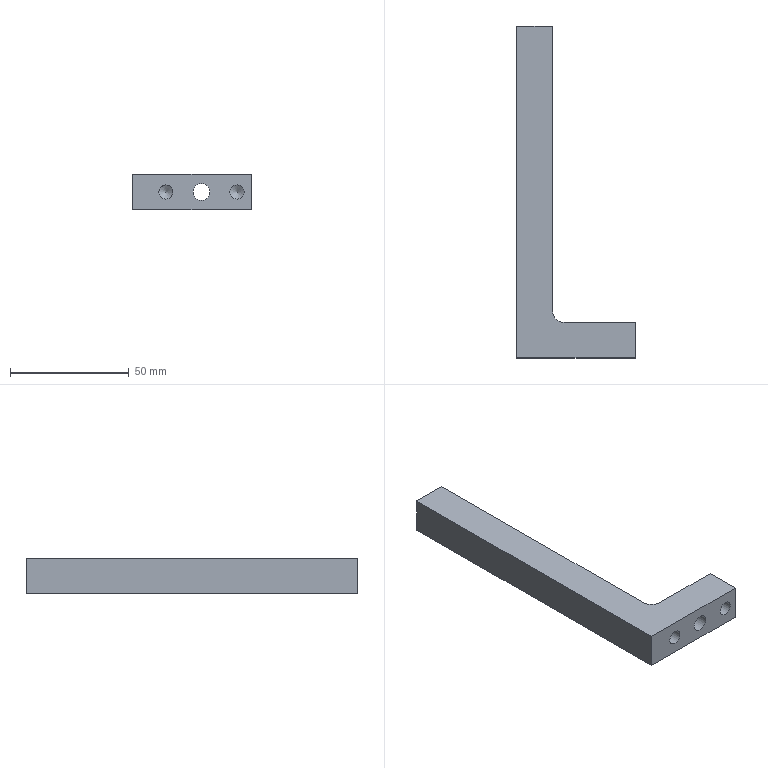Part | NX | features BREP 1 | 1 solid | 16 faces | box 50 x 140 x 15 mm | volume 37424 mm3 | plane 8 | cylinder 5 | cone 3 | commonest cylinder face diameters 6 x2 6.8 x1 7 x1 10 x1
STEP:
#1=CARTESIAN_POINT('',(15.,20.,0.));
#2=VERTEX_POINT('',#1);
#3=CARTESIAN_POINT('',(15.,140.,0.));
#4=VERTEX_POINT('',#3);
#5=CARTESIAN_POINT('',(15.,0.,0.));
#6=DIRECTION('',(0.,1.,0.));
#7=VECTOR('',#6,1000.);
#8=LINE('',#5,#7);
#9=EDGE_CURVE('',#2,#4,#8,.T.);
#10=ORIENTED_EDGE('',*,*,#9,.F.);
#11=CARTESIAN_POINT('',(20.,15.,0.));
#12=VERTEX_POINT('',#11);
#13=CARTESIAN_POINT('',(20.,20.,0.));
#14=DIRECTION('',(0.,0.,-1.));
#15=DIRECTION('',(1.,0.,0.));
#16=AXIS2_PLACEMENT_3D('',#13,#14,#15);
#17=CIRCLE('',#16,5.);
#18=EDGE_CURVE('',#12,#2,#17,.T.);
#19=ORIENTED_EDGE('',*,*,#18,.F.);
#20=CARTESIAN_POINT('',(50.,15.,0.));
#21=VERTEX_POINT('',#20);
#22=CARTESIAN_POINT('',(0.,15.,0.));
#23=DIRECTION('',(-1.,0.,0.));
#24=VECTOR('',#23,1000.);
#25=LINE('',#22,#24);
#26=EDGE_CURVE('',#21,#12,#25,.T.);
#27=ORIENTED_EDGE('',*,*,#26,.F.);
#28=CARTESIAN_POINT('',(50.,0.,0.));
#29=VERTEX_POINT('',#28);
#30=CARTESIAN_POINT('',(50.,0.,0.));
#31=DIRECTION('',(0.,1.,0.));
#32=VECTOR('',#31,1000.);
#33=LINE('',#30,#32);
#34=EDGE_CURVE('',#29,#21,#33,.T.);
#35=ORIENTED_EDGE('',*,*,#34,.F.);
#36=CARTESIAN_POINT('',(0.,0.,0.));
#37=VERTEX_POINT('',#36);
#38=CARTESIAN_POINT('',(0.,0.,0.));
#39=DIRECTION('',(1.,0.,0.));
#40=VECTOR('',#39,1000.);
#41=LINE('',#38,#40);
#42=EDGE_CURVE('',#37,#29,#41,.T.);
#43=ORIENTED_EDGE('',*,*,#42,.F.);
#44=CARTESIAN_POINT('',(0.,140.,0.));
#45=VERTEX_POINT('',#44);
#46=CARTESIAN_POINT('',(0.,0.,0.));
#47=DIRECTION('',(0.,-1.,0.));
#48=VECTOR('',#47,1000.);
#49=LINE('',#46,#48);
#50=EDGE_CURVE('',#45,#37,#49,.T.);
#51=ORIENTED_EDGE('',*,*,#50,.F.);
#52=CARTESIAN_POINT('',(0.,140.,0.));
#53=DIRECTION('',(-1.,0.,0.));
#54=VECTOR('',#53,1000.);
#55=LINE('',#52,#54);
#56=EDGE_CURVE('',#4,#45,#55,.T.);
#57=ORIENTED_EDGE('',*,*,#56,.F.);
#58=EDGE_LOOP('',(#10,#19,#27,#35,#43,#51,#57));
#59=FACE_BOUND('',#58,.T.);
#60=CARTESIAN_POINT('',(0.,0.,0.));
#61=DIRECTION('',(0.,0.,1.));
#62=DIRECTION('',(-1.,0.,0.));
#63=AXIS2_PLACEMENT_3D('',#60,#61,#62);
#64=PLANE('',#63);
#65=ADVANCED_FACE('',(#59),#64,.F.);
#66=CARTESIAN_POINT('',(0.,140.,15.));
#67=VERTEX_POINT('',#66);
#68=CARTESIAN_POINT('',(0.,140.,15.));
#69=DIRECTION('',(0.,0.,-1.));
#70=VECTOR('',#69,1000.);
#71=LINE('',#68,#70);
#72=EDGE_CURVE('',#67,#45,#71,.T.);
#73=ORIENTED_EDGE('',*,*,#72,.F.);
#74=CARTESIAN_POINT('',(15.,140.,15.));
#75=VERTEX_POINT('',#74);
#76=CARTESIAN_POINT('',(15.,140.,15.));
#77=DIRECTION('',(-1.,0.,0.));
#78=VECTOR('',#77,1000.);
#79=LINE('',#76,#78);
#80=EDGE_CURVE('',#75,#67,#79,.T.);
#81=ORIENTED_EDGE('',*,*,#80,.F.);
#82=CARTESIAN_POINT('',(15.,140.,15.));
#83=DIRECTION('',(0.,0.,1.));
#84=VECTOR('',#83,1000.);
#85=LINE('',#82,#84);
#86=EDGE_CURVE('',#4,#75,#85,.T.);
#87=ORIENTED_EDGE('',*,*,#86,.F.);
#88=ORIENTED_EDGE('',*,*,#56,.T.);
#89=EDGE_LOOP('',(#73,#81,#87,#88));
#90=FACE_BOUND('',#89,.T.);
#91=CARTESIAN_POINT('',(7.5,140.,10.9));
#92=VERTEX_POINT('',#91);
#93=CARTESIAN_POINT('',(7.5,140.,7.5));
#94=DIRECTION('',(0.,1.,0.));
#95=DIRECTION('',(0.,0.,1.));
#96=AXIS2_PLACEMENT_3D('',#93,#94,#95);
#97=CIRCLE('',#96,3.4);
#98=EDGE_CURVE('',#92,#92,#97,.T.);
#99=ORIENTED_EDGE('',*,*,#98,.F.);
#100=EDGE_LOOP('',(#99));
#101=FACE_BOUND('',#100,.T.);
#102=CARTESIAN_POINT('',(15.,140.,15.));
#103=DIRECTION('',(0.,-1.,0.));
#104=DIRECTION('',(0.,0.,1.));
#105=AXIS2_PLACEMENT_3D('',#102,#103,#104);
#106=PLANE('',#105);
#107=ADVANCED_FACE('',(#90,#101),#106,.F.);
#108=CARTESIAN_POINT('',(15.,20.,15.));
#109=VERTEX_POINT('',#108);
#110=CARTESIAN_POINT('',(15.,20.,15.));
#111=DIRECTION('',(0.,0.,1.));
#112=VECTOR('',#111,1000.);
#113=LINE('',#110,#112);
#114=EDGE_CURVE('',#2,#109,#113,.T.);
#115=ORIENTED_EDGE('',*,*,#114,.F.);
#116=ORIENTED_EDGE('',*,*,#9,.T.);
#117=ORIENTED_EDGE('',*,*,#86,.T.);
#118=CARTESIAN_POINT('',(15.,15.,15.));
#119=DIRECTION('',(0.,1.,0.));
#120=VECTOR('',#119,1000.);
#121=LINE('',#118,#120);
#122=EDGE_CURVE('',#109,#75,#121,.T.);
#123=ORIENTED_EDGE('',*,*,#122,.F.);
#124=EDGE_LOOP('',(#115,#116,#117,#123));
#125=FACE_BOUND('',#124,.T.);
#126=CARTESIAN_POINT('',(15.,15.,15.));
#127=DIRECTION('',(-1.,0.,0.));
#128=DIRECTION('',(0.,0.,-1.));
#129=AXIS2_PLACEMENT_3D('',#126,#127,#128);
#130=PLANE('',#129);
#131=ADVANCED_FACE('',(#125),#130,.F.);
#132=CARTESIAN_POINT('',(20.,15.,15.));
#133=VERTEX_POINT('',#132);
#134=CARTESIAN_POINT('',(20.,15.,15.));
#135=DIRECTION('',(0.,0.,1.));
#136=VECTOR('',#135,1000.);
#137=LINE('',#134,#136);
#138=EDGE_CURVE('',#12,#133,#137,.T.);
#139=ORIENTED_EDGE('',*,*,#138,.F.);
#140=ORIENTED_EDGE('',*,*,#18,.T.);
#141=ORIENTED_EDGE('',*,*,#114,.T.);
#142=CARTESIAN_POINT('',(20.,20.,15.));
#143=DIRECTION('',(0.,0.,-1.));
#144=DIRECTION('',(1.,0.,0.));
#145=AXIS2_PLACEMENT_3D('',#142,#143,#144);
#146=CIRCLE('',#145,5.);
#147=EDGE_CURVE('',#133,#109,#146,.T.);
#148=ORIENTED_EDGE('',*,*,#147,.F.);
#149=EDGE_LOOP('',(#139,#140,#141,#148));
#150=FACE_BOUND('',#149,.T.);
#151=CARTESIAN_POINT('',(20.,20.,15.));
#152=DIRECTION('',(0.,0.,1.));
#153=DIRECTION('',(-1.,0.,0.));
#154=AXIS2_PLACEMENT_3D('',#151,#152,#153);
#155=CYLINDRICAL_SURFACE('',#154,5.);
#156=ADVANCED_FACE('',(#150),#155,.F.);
#157=ORIENTED_EDGE('',*,*,#138,.T.);
#158=CARTESIAN_POINT('',(50.,15.,15.));
#159=VERTEX_POINT('',#158);
#160=CARTESIAN_POINT('',(50.,15.,15.));
#161=DIRECTION('',(-1.,0.,0.));
#162=VECTOR('',#161,1000.);
#163=LINE('',#160,#162);
#164=EDGE_CURVE('',#159,#133,#163,.T.);
#165=ORIENTED_EDGE('',*,*,#164,.F.);
#166=CARTESIAN_POINT('',(50.,15.,15.));
#167=DIRECTION('',(0.,0.,1.));
#168=VECTOR('',#167,1000.);
#169=LINE('',#166,#168);
#170=EDGE_CURVE('',#21,#159,#169,.T.);
#171=ORIENTED_EDGE('',*,*,#170,.F.);
#172=ORIENTED_EDGE('',*,*,#26,.T.);
#173=EDGE_LOOP('',(#157,#165,#171,#172));
#174=FACE_BOUND('',#173,.T.);
#175=CARTESIAN_POINT('',(29.,15.,4.));
#176=VERTEX_POINT('',#175);
#177=CARTESIAN_POINT('',(29.,15.,7.5));
#178=DIRECTION('',(0.,1.,0.));
#179=DIRECTION('',(0.,0.,-1.));
#180=AXIS2_PLACEMENT_3D('',#177,#178,#179);
#181=CIRCLE('',#180,3.5);
#182=EDGE_CURVE('',#176,#176,#181,.T.);
#183=ORIENTED_EDGE('',*,*,#182,.F.);
#184=EDGE_LOOP('',(#183));
#185=FACE_BOUND('',#184,.T.);
#186=CARTESIAN_POINT('',(50.,15.,15.));
#187=DIRECTION('',(0.,-1.,0.));
#188=DIRECTION('',(-1.,0.,0.));
#189=AXIS2_PLACEMENT_3D('',#186,#187,#188);
#190=PLANE('',#189);
#191=ADVANCED_FACE('',(#174,#185),#190,.F.);
#192=ORIENTED_EDGE('',*,*,#170,.T.);
#193=CARTESIAN_POINT('',(50.,0.,15.));
#194=VERTEX_POINT('',#193);
#195=CARTESIAN_POINT('',(50.,0.,15.));
#196=DIRECTION('',(0.,1.,0.));
#197=VECTOR('',#196,1000.);
#198=LINE('',#195,#197);
#199=EDGE_CURVE('',#194,#159,#198,.T.);
#200=ORIENTED_EDGE('',*,*,#199,.F.);
#201=CARTESIAN_POINT('',(50.,0.,15.));
#202=DIRECTION('',(0.,0.,1.));
#203=VECTOR('',#202,1000.);
#204=LINE('',#201,#203);
#205=EDGE_CURVE('',#29,#194,#204,.T.);
#206=ORIENTED_EDGE('',*,*,#205,.F.);
#207=ORIENTED_EDGE('',*,*,#34,.T.);
#208=EDGE_LOOP('',(#192,#200,#206,#207));
#209=FACE_BOUND('',#208,.T.);
#210=CARTESIAN_POINT('',(50.,0.,15.));
#211=DIRECTION('',(-1.,0.,0.));
#212=DIRECTION('',(0.,0.,-1.));
#213=AXIS2_PLACEMENT_3D('',#210,#211,#212);
#214=PLANE('',#213);
#215=ADVANCED_FACE('',(#209),#214,.F.);
#216=ORIENTED_EDGE('',*,*,#205,.T.);
#217=CARTESIAN_POINT('',(0.,0.,15.));
#218=VERTEX_POINT('',#217);
#219=CARTESIAN_POINT('',(0.,0.,15.));
#220=DIRECTION('',(1.,0.,0.));
#221=VECTOR('',#220,1000.);
#222=LINE('',#219,#221);
#223=EDGE_CURVE('',#218,#194,#222,.T.);
#224=ORIENTED_EDGE('',*,*,#223,.F.);
#225=CARTESIAN_POINT('',(0.,0.,15.));
#226=DIRECTION('',(0.,0.,1.));
#227=VECTOR('',#226,1000.);
#228=LINE('',#225,#227);
#229=EDGE_CURVE('',#37,#218,#228,.T.);
#230=ORIENTED_EDGE('',*,*,#229,.F.);
#231=ORIENTED_EDGE('',*,*,#42,.T.);
#232=EDGE_LOOP('',(#216,#224,#230,#231));
#233=FACE_BOUND('',#232,.T.);
#234=CARTESIAN_POINT('',(14.,0.,4.5));
#235=VERTEX_POINT('',#234);
#236=CARTESIAN_POINT('',(14.,0.,7.5));
#237=DIRECTION('',(0.,-1.,0.));
#238=DIRECTION('',(0.,0.,-1.));
#239=AXIS2_PLACEMENT_3D('',#236,#237,#238);
#240=CIRCLE('',#239,3.);
#241=EDGE_CURVE('',#235,#235,#240,.T.);
#242=ORIENTED_EDGE('',*,*,#241,.F.);
#243=EDGE_LOOP('',(#242));
#244=FACE_BOUND('',#243,.T.);
#245=CARTESIAN_POINT('',(44.,0.,4.5));
#246=VERTEX_POINT('',#245);
#247=CARTESIAN_POINT('',(44.,0.,7.5));
#248=DIRECTION('',(0.,-1.,0.));
#249=DIRECTION('',(0.,0.,-1.));
#250=AXIS2_PLACEMENT_3D('',#247,#248,#249);
#251=CIRCLE('',#250,3.);
#252=EDGE_CURVE('',#246,#246,#251,.T.);
#253=ORIENTED_EDGE('',*,*,#252,.F.);
#254=EDGE_LOOP('',(#253));
#255=FACE_BOUND('',#254,.T.);
#256=CARTESIAN_POINT('',(29.,0.,4.));
#257=VERTEX_POINT('',#256);
#258=CARTESIAN_POINT('',(29.,0.,7.5));
#259=DIRECTION('',(0.,-1.,0.));
#260=DIRECTION('',(0.,0.,-1.));
#261=AXIS2_PLACEMENT_3D('',#258,#259,#260);
#262=CIRCLE('',#261,3.5);
#263=EDGE_CURVE('',#257,#257,#262,.T.);
#264=ORIENTED_EDGE('',*,*,#263,.F.);
#265=EDGE_LOOP('',(#264));
#266=FACE_BOUND('',#265,.T.);
#267=CARTESIAN_POINT('',(0.,0.,15.));
#268=DIRECTION('',(0.,1.,0.));
#269=DIRECTION('',(0.,0.,-1.));
#270=AXIS2_PLACEMENT_3D('',#267,#268,#269);
#271=PLANE('',#270);
#272=ADVANCED_FACE('',(#233,#244,#255,#266),#271,.F.);
#273=ORIENTED_EDGE('',*,*,#229,.T.);
#274=CARTESIAN_POINT('',(0.,140.,15.));
#275=DIRECTION('',(0.,-1.,0.));
#276=VECTOR('',#275,1000.);
#277=LINE('',#274,#276);
#278=EDGE_CURVE('',#67,#218,#277,.T.);
#279=ORIENTED_EDGE('',*,*,#278,.F.);
#280=ORIENTED_EDGE('',*,*,#72,.T.);
#281=ORIENTED_EDGE('',*,*,#50,.T.);
#282=EDGE_LOOP('',(#273,#279,#280,#281));
#283=FACE_BOUND('',#282,.T.);
#284=CARTESIAN_POINT('',(0.,140.,15.));
#285=DIRECTION('',(1.,0.,0.));
#286=DIRECTION('',(0.,-1.,0.));
#287=AXIS2_PLACEMENT_3D('',#284,#285,#286);
#288=PLANE('',#287);
#289=ADVANCED_FACE('',(#283),#288,.F.);
#290=ORIENTED_EDGE('',*,*,#147,.T.);
#291=ORIENTED_EDGE('',*,*,#122,.T.);
#292=ORIENTED_EDGE('',*,*,#80,.T.);
#293=ORIENTED_EDGE('',*,*,#278,.T.);
#294=ORIENTED_EDGE('',*,*,#223,.T.);
#295=ORIENTED_EDGE('',*,*,#199,.T.);
#296=ORIENTED_EDGE('',*,*,#164,.T.);
#297=EDGE_LOOP('',(#290,#291,#292,#293,#294,#295,#296));
#298=FACE_BOUND('',#297,.T.);
#299=CARTESIAN_POINT('',(0.,0.,15.));
#300=DIRECTION('',(0.,0.,1.));
#301=DIRECTION('',(-1.,0.,0.));
#302=AXIS2_PLACEMENT_3D('',#299,#300,#301);
#303=PLANE('',#302);
#304=ADVANCED_FACE('',(#298),#303,.T.);
#305=CARTESIAN_POINT('',(7.5,120.25,10.9));
#306=VERTEX_POINT('',#305);
#307=CARTESIAN_POINT('',(7.5,120.25,7.5));
#308=DIRECTION('',(0.,1.,0.));
#309=DIRECTION('',(0.,0.,1.));
#310=AXIS2_PLACEMENT_3D('',#307,#308,#309);
#311=CIRCLE('',#310,3.4);
#312=EDGE_CURVE('',#306,#306,#311,.T.);
#313=ORIENTED_EDGE('',*,*,#312,.F.);
#314=EDGE_LOOP('',(#313));
#315=FACE_BOUND('',#314,.T.);
#316=ORIENTED_EDGE('',*,*,#98,.T.);
#317=EDGE_LOOP('',(#316));
#318=FACE_BOUND('',#317,.T.);
#319=CARTESIAN_POINT('',(7.5,140.,7.5));
#320=DIRECTION('',(0.,1.,0.));
#321=DIRECTION('',(0.,0.,-1.));
#322=AXIS2_PLACEMENT_3D('',#319,#320,#321);
#323=CYLINDRICAL_SURFACE('',#322,3.4);
#324=ADVANCED_FACE('',(#315,#318),#323,.F.);
#325=ORIENTED_EDGE('',*,*,#182,.T.);
#326=EDGE_LOOP('',(#325));
#327=FACE_BOUND('',#326,.T.);
#328=ORIENTED_EDGE('',*,*,#263,.T.);
#329=EDGE_LOOP('',(#328));
#330=FACE_BOUND('',#329,.T.);
#331=CARTESIAN_POINT('',(29.,0.,7.5));
#332=DIRECTION('',(0.,-1.,0.));
#333=DIRECTION('',(0.,0.,1.));
#334=AXIS2_PLACEMENT_3D('',#331,#332,#333);
#335=CYLINDRICAL_SURFACE('',#334,3.5);
#336=ADVANCED_FACE('',(#327,#330),#335,.F.);
#337=CARTESIAN_POINT('',(14.,12.,4.5));
#338=VERTEX_POINT('',#337);
#339=CARTESIAN_POINT('',(14.,12.,7.5));
#340=DIRECTION('',(0.,-1.,0.));
#341=DIRECTION('',(0.,0.,-1.));
#342=AXIS2_PLACEMENT_3D('',#339,#340,#341);
#343=CIRCLE('',#342,3.);
#344=EDGE_CURVE('',#338,#338,#343,.T.);
#345=ORIENTED_EDGE('',*,*,#344,.F.);
#346=EDGE_LOOP('',(#345));
#347=FACE_BOUND('',#346,.T.);
#348=ORIENTED_EDGE('',*,*,#241,.T.);
#349=EDGE_LOOP('',(#348));
#350=FACE_BOUND('',#349,.T.);
#351=CARTESIAN_POINT('',(14.,0.,7.5));
#352=DIRECTION('',(0.,-1.,0.));
#353=DIRECTION('',(0.,0.,1.));
#354=AXIS2_PLACEMENT_3D('',#351,#352,#353);
#355=CYLINDRICAL_SURFACE('',#354,3.);
#356=ADVANCED_FACE('',(#347,#350),#355,.F.);
#357=CARTESIAN_POINT('',(44.,12.,4.5));
#358=VERTEX_POINT('',#357);
#359=CARTESIAN_POINT('',(44.,12.,7.5));
#360=DIRECTION('',(0.,-1.,0.));
#361=DIRECTION('',(0.,0.,-1.));
#362=AXIS2_PLACEMENT_3D('',#359,#360,#361);
#363=CIRCLE('',#362,3.);
#364=EDGE_CURVE('',#358,#358,#363,.T.);
#365=ORIENTED_EDGE('',*,*,#364,.F.);
#366=EDGE_LOOP('',(#365));
#367=FACE_BOUND('',#366,.T.);
#368=ORIENTED_EDGE('',*,*,#252,.T.);
#369=EDGE_LOOP('',(#368));
#370=FACE_BOUND('',#369,.T.);
#371=CARTESIAN_POINT('',(44.,0.,7.5));
#372=DIRECTION('',(0.,-1.,0.));
#373=DIRECTION('',(0.,0.,1.));
#374=AXIS2_PLACEMENT_3D('',#371,#372,#373);
#375=CYLINDRICAL_SURFACE('',#374,3.);
#376=ADVANCED_FACE('',(#367,#370),#375,.F.);
#377=CARTESIAN_POINT('',(7.5,118.207,7.5));
#378=VERTEX_POINT('',#377);
#379=VERTEX_LOOP('',#378);
#380=FACE_BOUND('',#379,.T.);
#381=ORIENTED_EDGE('',*,*,#312,.T.);
#382=EDGE_LOOP('',(#381));
#383=FACE_BOUND('',#382,.T.);
#384=CARTESIAN_POINT('',(7.5,120.25,7.5));
#385=DIRECTION('',(0.,1.,0.));
#386=DIRECTION('',(0.,0.,-1.));
#387=AXIS2_PLACEMENT_3D('',#384,#385,#386);
#388=CONICAL_SURFACE('',#387,3.4,1.03);
#389=ADVANCED_FACE('',(#380,#383),#388,.F.);
#390=CARTESIAN_POINT('',(14.,13.803,7.5));
#391=VERTEX_POINT('',#390);
#392=VERTEX_LOOP('',#391);
#393=FACE_BOUND('',#392,.T.);
#394=ORIENTED_EDGE('',*,*,#344,.T.);
#395=EDGE_LOOP('',(#394));
#396=FACE_BOUND('',#395,.T.);
#397=CARTESIAN_POINT('',(14.,12.,7.5));
#398=DIRECTION('',(0.,-1.,0.));
#399=DIRECTION('',(-1.,0.,0.));
#400=AXIS2_PLACEMENT_3D('',#397,#398,#399);
#401=CONICAL_SURFACE('',#400,3.,1.03);
#402=ADVANCED_FACE('',(#393,#396),#401,.F.);
#403=CARTESIAN_POINT('',(44.,13.803,7.5));
#404=VERTEX_POINT('',#403);
#405=VERTEX_LOOP('',#404);
#406=FACE_BOUND('',#405,.T.);
#407=ORIENTED_EDGE('',*,*,#364,.T.);
#408=EDGE_LOOP('',(#407));
#409=FACE_BOUND('',#408,.T.);
#410=CARTESIAN_POINT('',(44.,12.,7.5));
#411=DIRECTION('',(0.,-1.,0.));
#412=DIRECTION('',(0.,0.,1.));
#413=AXIS2_PLACEMENT_3D('',#410,#411,#412);
#414=CONICAL_SURFACE('',#413,3.,1.03);
#415=ADVANCED_FACE('',(#406,#409),#414,.F.);
#416=CLOSED_SHELL('',(#65,#107,#131,#156,#191,#215,#272,#289,#304,#324,#336,#356,#376,#389,#402,#415));
#417=MANIFOLD_SOLID_BREP('',#416);
#418=(LENGTH_UNIT()NAMED_UNIT(*)SI_UNIT(.MILLI.,.METRE.));
#419=UNCERTAINTY_MEASURE_WITH_UNIT(LENGTH_MEASURE(0.00001),#418,'','');
#420=(NAMED_UNIT(*)PLANE_ANGLE_UNIT()SI_UNIT($,.RADIAN.));
#421=(NAMED_UNIT(*)SI_UNIT($,.STERADIAN.)SOLID_ANGLE_UNIT());
#422=(GEOMETRIC_REPRESENTATION_CONTEXT(3)GLOBAL_UNCERTAINTY_ASSIGNED_CONTEXT((#419))GLOBAL_UNIT_ASSIGNED_CONTEXT((#418,#420,#421))REPRESENTATION_CONTEXT('',''));
#423=ADVANCED_BREP_SHAPE_REPRESENTATION('',(#417),#422);